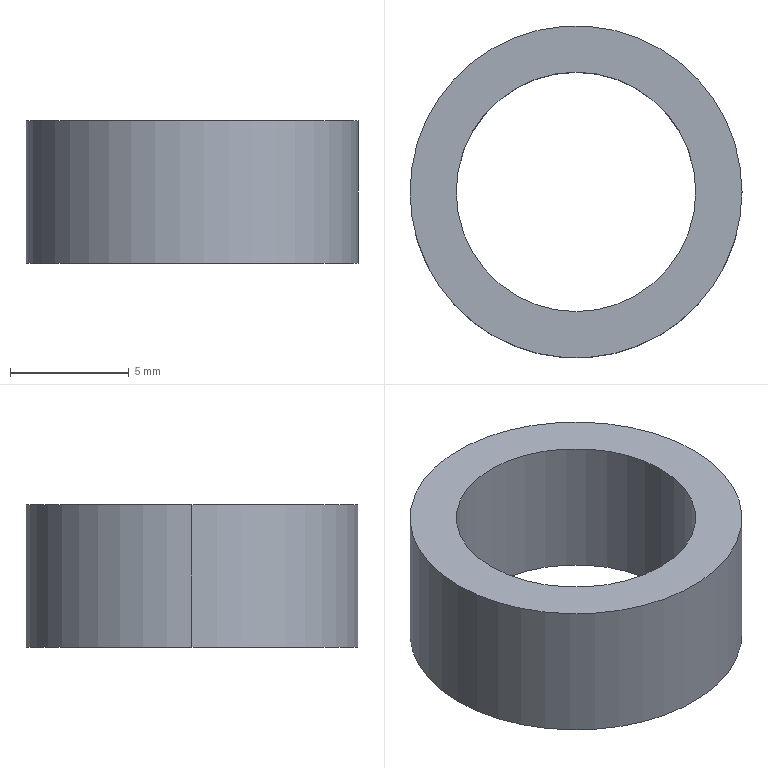Part | NX | features BREP 1 | 1 solid | 6 faces | box 14 x 14 x 6 mm | volume 442.917 mm3 | cylinder 4 | plane 2 | commonest cylinder face diameters 10.1 x2 14 x2
STEP:
#1=CARTESIAN_POINT('',(5.05,0.,6.));
#2=VERTEX_POINT('',#1);
#3=CARTESIAN_POINT('',(5.05,0.,0.));
#4=VERTEX_POINT('',#3);
#5=CARTESIAN_POINT('',(5.05,0.,6.));
#6=DIRECTION('',(0.,0.,-1.));
#7=VECTOR('',#6,1000.);
#8=LINE('',#5,#7);
#9=EDGE_CURVE('',#2,#4,#8,.T.);
#10=ORIENTED_EDGE('',*,*,#9,.F.);
#11=CARTESIAN_POINT('',(-5.05,0.,6.));
#12=VERTEX_POINT('',#11);
#13=CARTESIAN_POINT('',(0.,0.,6.));
#14=DIRECTION('',(0.,0.,1.));
#15=DIRECTION('',(1.,0.,0.));
#16=AXIS2_PLACEMENT_3D('',#13,#14,#15);
#17=CIRCLE('',#16,5.05);
#18=EDGE_CURVE('',#2,#12,#17,.T.);
#19=ORIENTED_EDGE('',*,*,#18,.T.);
#20=CARTESIAN_POINT('',(-5.05,0.,0.));
#21=VERTEX_POINT('',#20);
#22=CARTESIAN_POINT('',(-5.05,0.,6.));
#23=DIRECTION('',(0.,0.,-1.));
#24=VECTOR('',#23,1000.);
#25=LINE('',#22,#24);
#26=EDGE_CURVE('',#12,#21,#25,.T.);
#27=ORIENTED_EDGE('',*,*,#26,.T.);
#28=CARTESIAN_POINT('',(0.,0.,0.));
#29=DIRECTION('',(0.,0.,1.));
#30=DIRECTION('',(1.,0.,0.));
#31=AXIS2_PLACEMENT_3D('',#28,#29,#30);
#32=CIRCLE('',#31,5.05);
#33=EDGE_CURVE('',#4,#21,#32,.T.);
#34=ORIENTED_EDGE('',*,*,#33,.F.);
#35=EDGE_LOOP('',(#10,#19,#27,#34));
#36=FACE_BOUND('',#35,.T.);
#37=CARTESIAN_POINT('',(0.,0.,6.));
#38=DIRECTION('',(0.,0.,-1.));
#39=DIRECTION('',(-1.,0.,0.));
#40=AXIS2_PLACEMENT_3D('',#37,#38,#39);
#41=CYLINDRICAL_SURFACE('',#40,5.05);
#42=ADVANCED_FACE('',(#36),#41,.F.);
#43=CARTESIAN_POINT('',(7.,0.,6.));
#44=VERTEX_POINT('',#43);
#45=CARTESIAN_POINT('',(7.,0.,0.));
#46=VERTEX_POINT('',#45);
#47=CARTESIAN_POINT('',(7.,0.,6.));
#48=DIRECTION('',(0.,0.,-1.));
#49=VECTOR('',#48,1000.);
#50=LINE('',#47,#49);
#51=EDGE_CURVE('',#44,#46,#50,.T.);
#52=ORIENTED_EDGE('',*,*,#51,.F.);
#53=CARTESIAN_POINT('',(-7.,0.,6.));
#54=VERTEX_POINT('',#53);
#55=CARTESIAN_POINT('',(0.,0.,6.));
#56=DIRECTION('',(0.,0.,1.));
#57=DIRECTION('',(1.,0.,0.));
#58=AXIS2_PLACEMENT_3D('',#55,#56,#57);
#59=CIRCLE('',#58,7.);
#60=EDGE_CURVE('',#54,#44,#59,.T.);
#61=ORIENTED_EDGE('',*,*,#60,.F.);
#62=CARTESIAN_POINT('',(-7.,0.,0.));
#63=VERTEX_POINT('',#62);
#64=CARTESIAN_POINT('',(-7.,0.,6.));
#65=DIRECTION('',(0.,0.,-1.));
#66=VECTOR('',#65,1000.);
#67=LINE('',#64,#66);
#68=EDGE_CURVE('',#54,#63,#67,.T.);
#69=ORIENTED_EDGE('',*,*,#68,.T.);
#70=CARTESIAN_POINT('',(0.,0.,0.));
#71=DIRECTION('',(0.,0.,1.));
#72=DIRECTION('',(1.,0.,0.));
#73=AXIS2_PLACEMENT_3D('',#70,#71,#72);
#74=CIRCLE('',#73,7.);
#75=EDGE_CURVE('',#63,#46,#74,.T.);
#76=ORIENTED_EDGE('',*,*,#75,.T.);
#77=EDGE_LOOP('',(#52,#61,#69,#76));
#78=FACE_BOUND('',#77,.T.);
#79=CARTESIAN_POINT('',(0.,0.,6.));
#80=DIRECTION('',(0.,0.,-1.));
#81=DIRECTION('',(-1.,0.,0.));
#82=AXIS2_PLACEMENT_3D('',#79,#80,#81);
#83=CYLINDRICAL_SURFACE('',#82,7.);
#84=ADVANCED_FACE('',(#78),#83,.T.);
#85=CARTESIAN_POINT('',(0.,0.,0.));
#86=DIRECTION('',(0.,0.,1.));
#87=DIRECTION('',(1.,0.,0.));
#88=AXIS2_PLACEMENT_3D('',#85,#86,#87);
#89=CIRCLE('',#88,5.05);
#90=EDGE_CURVE('',#21,#4,#89,.T.);
#91=ORIENTED_EDGE('',*,*,#90,.T.);
#92=ORIENTED_EDGE('',*,*,#33,.T.);
#93=EDGE_LOOP('',(#91,#92));
#94=FACE_BOUND('',#93,.T.);
#95=ORIENTED_EDGE('',*,*,#75,.F.);
#96=CARTESIAN_POINT('',(0.,0.,0.));
#97=DIRECTION('',(0.,0.,1.));
#98=DIRECTION('',(1.,0.,0.));
#99=AXIS2_PLACEMENT_3D('',#96,#97,#98);
#100=CIRCLE('',#99,7.);
#101=EDGE_CURVE('',#46,#63,#100,.T.);
#102=ORIENTED_EDGE('',*,*,#101,.F.);
#103=EDGE_LOOP('',(#95,#102));
#104=FACE_BOUND('',#103,.T.);
#105=CARTESIAN_POINT('',(0.,0.,0.));
#106=DIRECTION('',(0.,0.,1.));
#107=DIRECTION('',(1.,0.,0.));
#108=AXIS2_PLACEMENT_3D('',#105,#106,#107);
#109=PLANE('',#108);
#110=ADVANCED_FACE('',(#94,#104),#109,.F.);
#111=CARTESIAN_POINT('',(0.,0.,6.));
#112=DIRECTION('',(0.,0.,1.));
#113=DIRECTION('',(1.,0.,0.));
#114=AXIS2_PLACEMENT_3D('',#111,#112,#113);
#115=CIRCLE('',#114,5.05);
#116=EDGE_CURVE('',#12,#2,#115,.T.);
#117=ORIENTED_EDGE('',*,*,#116,.F.);
#118=ORIENTED_EDGE('',*,*,#18,.F.);
#119=EDGE_LOOP('',(#117,#118));
#120=FACE_BOUND('',#119,.T.);
#121=ORIENTED_EDGE('',*,*,#60,.T.);
#122=CARTESIAN_POINT('',(0.,0.,6.));
#123=DIRECTION('',(0.,0.,1.));
#124=DIRECTION('',(1.,0.,0.));
#125=AXIS2_PLACEMENT_3D('',#122,#123,#124);
#126=CIRCLE('',#125,7.);
#127=EDGE_CURVE('',#44,#54,#126,.T.);
#128=ORIENTED_EDGE('',*,*,#127,.T.);
#129=EDGE_LOOP('',(#121,#128));
#130=FACE_BOUND('',#129,.T.);
#131=CARTESIAN_POINT('',(0.,0.,6.));
#132=DIRECTION('',(0.,0.,1.));
#133=DIRECTION('',(1.,0.,0.));
#134=AXIS2_PLACEMENT_3D('',#131,#132,#133);
#135=PLANE('',#134);
#136=ADVANCED_FACE('',(#120,#130),#135,.T.);
#137=ORIENTED_EDGE('',*,*,#127,.F.);
#138=ORIENTED_EDGE('',*,*,#51,.T.);
#139=ORIENTED_EDGE('',*,*,#101,.T.);
#140=ORIENTED_EDGE('',*,*,#68,.F.);
#141=EDGE_LOOP('',(#137,#138,#139,#140));
#142=FACE_BOUND('',#141,.T.);
#143=CARTESIAN_POINT('',(0.,0.,6.));
#144=DIRECTION('',(0.,0.,-1.));
#145=DIRECTION('',(-1.,0.,0.));
#146=AXIS2_PLACEMENT_3D('',#143,#144,#145);
#147=CYLINDRICAL_SURFACE('',#146,7.);
#148=ADVANCED_FACE('',(#142),#147,.T.);
#149=ORIENTED_EDGE('',*,*,#116,.T.);
#150=ORIENTED_EDGE('',*,*,#9,.T.);
#151=ORIENTED_EDGE('',*,*,#90,.F.);
#152=ORIENTED_EDGE('',*,*,#26,.F.);
#153=EDGE_LOOP('',(#149,#150,#151,#152));
#154=FACE_BOUND('',#153,.T.);
#155=CARTESIAN_POINT('',(0.,0.,6.));
#156=DIRECTION('',(0.,0.,-1.));
#157=DIRECTION('',(-1.,0.,0.));
#158=AXIS2_PLACEMENT_3D('',#155,#156,#157);
#159=CYLINDRICAL_SURFACE('',#158,5.05);
#160=ADVANCED_FACE('',(#154),#159,.F.);
#161=CLOSED_SHELL('',(#42,#84,#110,#136,#148,#160));
#162=MANIFOLD_SOLID_BREP('',#161);
#163=(LENGTH_UNIT()NAMED_UNIT(*)SI_UNIT(.MILLI.,.METRE.));
#164=UNCERTAINTY_MEASURE_WITH_UNIT(LENGTH_MEASURE(0.00001),#163,'','');
#165=(NAMED_UNIT(*)PLANE_ANGLE_UNIT()SI_UNIT($,.RADIAN.));
#166=(NAMED_UNIT(*)SI_UNIT($,.STERADIAN.)SOLID_ANGLE_UNIT());
#167=(GEOMETRIC_REPRESENTATION_CONTEXT(3)GLOBAL_UNCERTAINTY_ASSIGNED_CONTEXT((#164))GLOBAL_UNIT_ASSIGNED_CONTEXT((#163,#165,#166))REPRESENTATION_CONTEXT('',''));
#168=ADVANCED_BREP_SHAPE_REPRESENTATION('',(#162),#167);